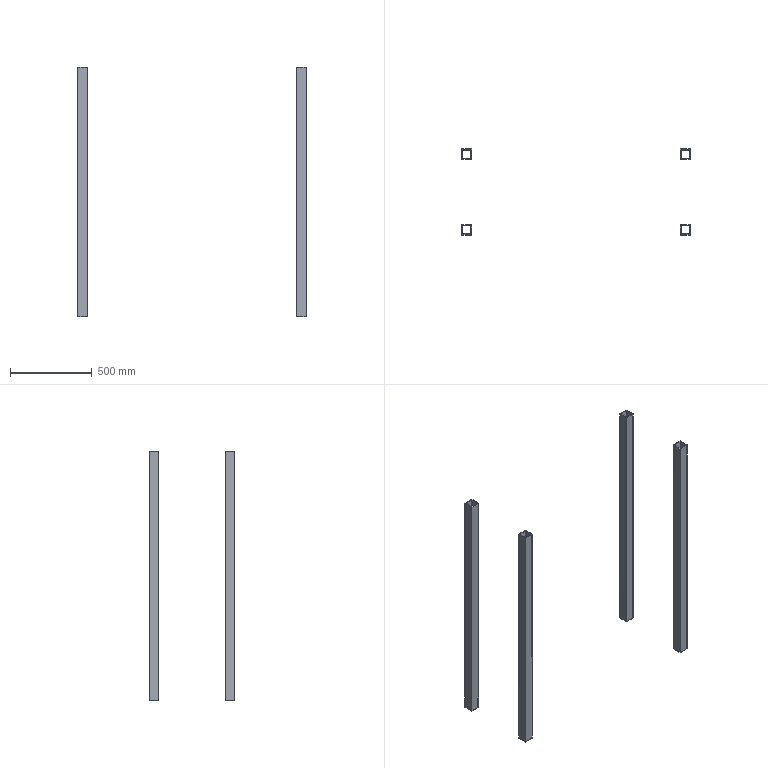Part | STEP file | ASND-0110-E63-HLTP01标准Lower机架-03 | 4 solids | 64 faces | box 1400 x 525 x 1530 mm | volume 5482578 mm3 | plane 40 | cylinder 24 | commonest cylinder face diameters 5 x24